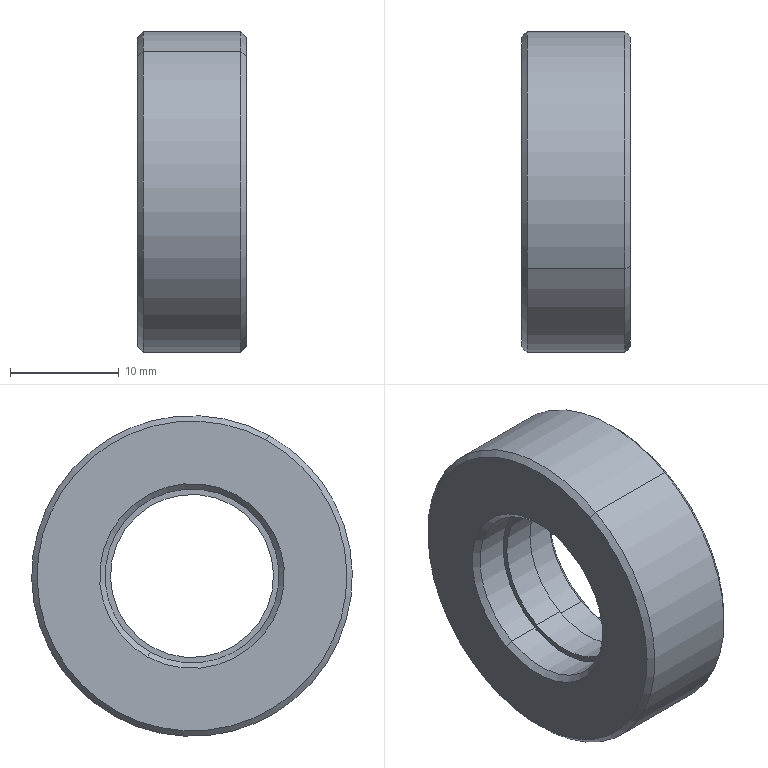Part | STEP file | DOWEL DISC(DOWEL DISC(Φ29.5×
10)) | 1 solid | 20 faces | box 10 x 29.5 x 29.5 mm | volume 4862 mm3 | cylinder 8 | cone 8 | plane 4 | commonest cylinder face diameters 16 x4 15 x2 29.5 x2